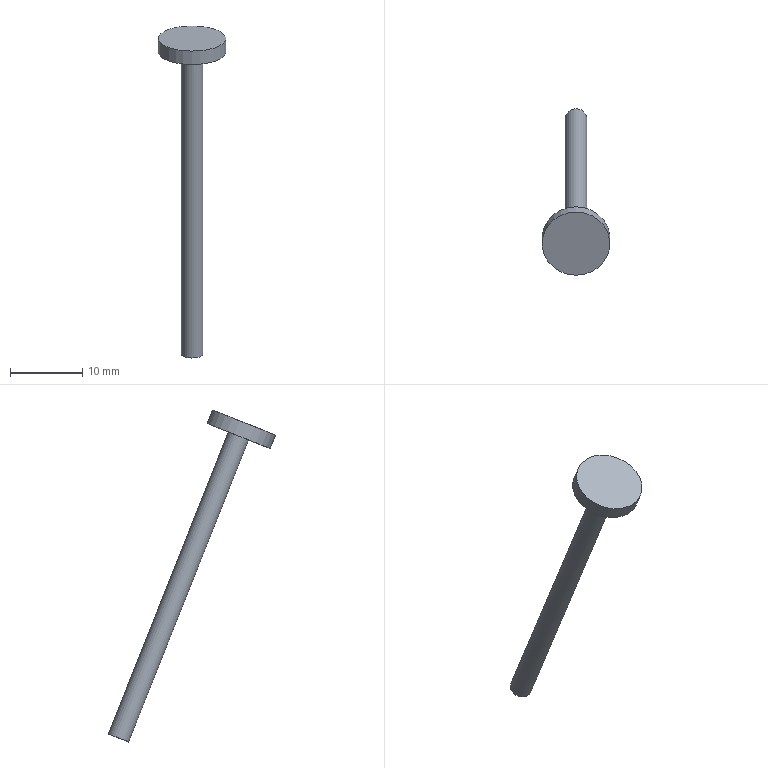Part | STEP file | Revolve1 | 1 solid | 5 faces | box 9.4 x 23.118 x 45.968 mm | volume 456.882 mm3 | plane 3 | cylinder 2 | commonest cylinder face diameters 3 x1 9.4 x1
STEP:
#1=CARTESIAN_POINT('',(0.,0.,0.));
#2=DIRECTION('',(0.,0.,1.));
#3=DIRECTION('',(1.,0.,0.));
#4=AXIS2_PLACEMENT_3D('',#1,#2,#3);
#5=CARTESIAN_POINT('',(140.817,148.133,-138.172));
#6=VERTEX_POINT('',#5);
#7=CARTESIAN_POINT('',(140.817,131.516,-96.352));
#8=VERTEX_POINT('',#7);
#9=CARTESIAN_POINT('',(140.817,148.133,-138.172));
#10=DIRECTION('',(0.,-0.3693,0.9293));
#11=VECTOR('',#10,1.);
#12=LINE('',#9,#11);
#13=CARTESIAN_POINT('',(140.797,130.122,-96.906));
#14=DIRECTION('',(0.,0.3693,-0.9293));
#15=DIRECTION('',(0.01361,0.9292,0.3692));
#16=AXIS2_PLACEMENT_3D('',#13,#14,#15);
#17=CYLINDRICAL_SURFACE('',#16,1.5);
#18=CARTESIAN_POINT('',(0.000000001,45.));
#19=DIRECTION('',(0.,-1.));
#20=VECTOR('',#19,1.);
#21=LINE('',#18,#20);
#22=(GEOMETRIC_REPRESENTATION_CONTEXT(2)PARAMETRIC_REPRESENTATION_CONTEXT()REPRESENTATION_CONTEXT('',''));
#23=DEFINITIONAL_REPRESENTATION('',(#21),#22);
#24=PCURVE('',#17,#23);
#25=CARTESIAN_POINT('',(6.283,45.));
#26=DIRECTION('',(0.,-1.));
#27=VECTOR('',#26,1.);
#28=LINE('',#25,#27);
#29=(GEOMETRIC_REPRESENTATION_CONTEXT(2)PARAMETRIC_REPRESENTATION_CONTEXT()REPRESENTATION_CONTEXT('',''));
#30=DEFINITIONAL_REPRESENTATION('',(#28),#29);
#31=PCURVE('',#17,#30);
#32=SEAM_CURVE('',#12,(#24,#31),.PCURVE_S1.);
#33=EDGE_CURVE('',#6,#8,#32,.T.);
#34=ORIENTED_EDGE('',*,*,#33,.T.);
#35=CARTESIAN_POINT('',(140.797,130.122,-96.906));
#36=DIRECTION('',(0.,0.3693,-0.9293));
#37=DIRECTION('',(0.01361,0.9292,0.3692));
#38=AXIS2_PLACEMENT_3D('',#35,#36,#37);
#39=CIRCLE('',#38,1.5);
#40=CARTESIAN_POINT('',(0.,0.));
#41=DIRECTION('',(1.,0.));
#42=VECTOR('',#41,1.);
#43=LINE('',#40,#42);
#44=(GEOMETRIC_REPRESENTATION_CONTEXT(2)PARAMETRIC_REPRESENTATION_CONTEXT()REPRESENTATION_CONTEXT('',''));
#45=DEFINITIONAL_REPRESENTATION('',(#43),#44);
#46=PCURVE('',#17,#45);
#47=CARTESIAN_POINT('',(140.797,130.122,-96.906));
#48=DIRECTION('',(0.,-0.3693,0.9293));
#49=DIRECTION('',(-0.01361,-0.9292,-0.3692));
#50=AXIS2_PLACEMENT_3D('',#47,#48,#49);
#51=PLANE('',#50);
#52=CARTESIAN_POINT('',(-1.5,0.));
#53=CARTESIAN_POINT('',(-1.5,2.598));
#54=CARTESIAN_POINT('',(0.75,1.299));
#55=CARTESIAN_POINT('',(3.,0.));
#56=CARTESIAN_POINT('',(0.75,-1.299));
#57=CARTESIAN_POINT('',(-1.5,-2.598));
#58=CARTESIAN_POINT('',(-1.5,0.));
#59=(BOUNDED_CURVE()B_SPLINE_CURVE(2,(#52,#53,#54,#55,#56,#57,#58),.UNSPECIFIED.,.T.,.F.)B_SPLINE_CURVE_WITH_KNOTS((1,2,2,2,2,1),(-2.094,0.,2.094,4.189,6.283,8.378),.UNSPECIFIED.)CURVE()GEOMETRIC_REPRESENTATION_ITEM()RATIONAL_B_SPLINE_CURVE((1.,0.5,1.,0.5,1.,0.5,1.))REPRESENTATION_ITEM(''));
#60=(GEOMETRIC_REPRESENTATION_CONTEXT(2)PARAMETRIC_REPRESENTATION_CONTEXT()REPRESENTATION_CONTEXT('',''));
#61=DEFINITIONAL_REPRESENTATION('',(#59),#60);
#62=PCURVE('',#51,#61);
#63=SURFACE_CURVE('',#39,(#46,#62),.PCURVE_S1.);
#64=EDGE_CURVE('',#8,#8,#63,.T.);
#65=ORIENTED_EDGE('',*,*,#64,.T.);
#66=ORIENTED_EDGE('',*,*,#33,.F.);
#67=CARTESIAN_POINT('',(140.797,146.739,-138.726));
#68=DIRECTION('',(0.,-0.3693,0.9293));
#69=DIRECTION('',(0.01361,0.9292,0.3692));
#70=AXIS2_PLACEMENT_3D('',#67,#68,#69);
#71=CIRCLE('',#70,1.5);
#72=CARTESIAN_POINT('',(6.283,45.));
#73=DIRECTION('',(-1.,0.));
#74=VECTOR('',#73,1.);
#75=LINE('',#72,#74);
#76=(GEOMETRIC_REPRESENTATION_CONTEXT(2)PARAMETRIC_REPRESENTATION_CONTEXT()REPRESENTATION_CONTEXT('',''));
#77=DEFINITIONAL_REPRESENTATION('',(#75),#76);
#78=PCURVE('',#17,#77);
#79=CARTESIAN_POINT('',(140.797,146.739,-138.726));
#80=DIRECTION('',(0.,-0.3693,0.9293));
#81=DIRECTION('',(-0.01361,-0.9292,-0.3692));
#82=AXIS2_PLACEMENT_3D('',#79,#80,#81);
#83=PLANE('',#82);
#84=CARTESIAN_POINT('',(0.,0.));
#85=DIRECTION('',(-1.,0.));
#86=AXIS2_PLACEMENT_2D('',#84,#85);
#87=CIRCLE('',#86,1.5);
#88=(GEOMETRIC_REPRESENTATION_CONTEXT(2)PARAMETRIC_REPRESENTATION_CONTEXT()REPRESENTATION_CONTEXT('',''));
#89=DEFINITIONAL_REPRESENTATION('',(#87),#88);
#90=PCURVE('',#83,#89);
#91=SURFACE_CURVE('',#71,(#78,#90),.PCURVE_S1.);
#92=EDGE_CURVE('',#6,#6,#91,.T.);
#93=ORIENTED_EDGE('',*,*,#92,.T.);
#94=EDGE_LOOP('',(#34,#65,#66,#93));
#95=FACE_BOUND('',#94,.T.);
#96=ADVANCED_FACE('',(#95),#17,.T.);
#97=CARTESIAN_POINT('',(140.861,134.489,-95.171));
#98=VERTEX_POINT('',#97);
#99=CARTESIAN_POINT('',(140.861,133.751,-93.312));
#100=VERTEX_POINT('',#99);
#101=CARTESIAN_POINT('',(140.861,134.489,-95.171));
#102=DIRECTION('',(0.,-0.3693,0.9293));
#103=VECTOR('',#102,1.);
#104=LINE('',#101,#103);
#105=CARTESIAN_POINT('',(140.797,129.383,-95.048));
#106=DIRECTION('',(0.,0.3693,-0.9293));
#107=DIRECTION('',(0.01361,0.9292,0.3692));
#108=AXIS2_PLACEMENT_3D('',#105,#106,#107);
#109=CYLINDRICAL_SURFACE('',#108,4.7);
#110=CARTESIAN_POINT('',(0.,2.));
#111=DIRECTION('',(0.,-1.));
#112=VECTOR('',#111,1.);
#113=LINE('',#110,#112);
#114=(GEOMETRIC_REPRESENTATION_CONTEXT(2)PARAMETRIC_REPRESENTATION_CONTEXT()REPRESENTATION_CONTEXT('',''));
#115=DEFINITIONAL_REPRESENTATION('',(#113),#114);
#116=PCURVE('',#109,#115);
#117=CARTESIAN_POINT('',(6.283,2.));
#118=DIRECTION('',(0.,-1.));
#119=VECTOR('',#118,1.);
#120=LINE('',#117,#119);
#121=(GEOMETRIC_REPRESENTATION_CONTEXT(2)PARAMETRIC_REPRESENTATION_CONTEXT()REPRESENTATION_CONTEXT('',''));
#122=DEFINITIONAL_REPRESENTATION('',(#120),#121);
#123=PCURVE('',#109,#122);
#124=SEAM_CURVE('',#104,(#116,#123),.PCURVE_S1.);
#125=EDGE_CURVE('',#98,#100,#124,.T.);
#126=ORIENTED_EDGE('',*,*,#125,.T.);
#127=CARTESIAN_POINT('',(140.797,129.383,-95.048));
#128=DIRECTION('',(0.,0.3693,-0.9293));
#129=DIRECTION('',(0.01361,0.9292,0.3692));
#130=AXIS2_PLACEMENT_3D('',#127,#128,#129);
#131=CIRCLE('',#130,4.7);
#132=CARTESIAN_POINT('',(0.,0.));
#133=DIRECTION('',(1.,0.));
#134=VECTOR('',#133,1.);
#135=LINE('',#132,#134);
#136=(GEOMETRIC_REPRESENTATION_CONTEXT(2)PARAMETRIC_REPRESENTATION_CONTEXT()REPRESENTATION_CONTEXT('',''));
#137=DEFINITIONAL_REPRESENTATION('',(#135),#136);
#138=PCURVE('',#109,#137);
#139=CARTESIAN_POINT('',(140.797,129.383,-95.048));
#140=DIRECTION('',(0.,0.3693,-0.9293));
#141=DIRECTION('',(0.01361,0.9292,0.3692));
#142=AXIS2_PLACEMENT_3D('',#139,#140,#141);
#143=PLANE('',#142);
#144=CARTESIAN_POINT('',(0.,0.));
#145=DIRECTION('',(1.,0.));
#146=AXIS2_PLACEMENT_2D('',#144,#145);
#147=CIRCLE('',#146,4.7);
#148=(GEOMETRIC_REPRESENTATION_CONTEXT(2)PARAMETRIC_REPRESENTATION_CONTEXT()REPRESENTATION_CONTEXT('',''));
#149=DEFINITIONAL_REPRESENTATION('',(#147),#148);
#150=PCURVE('',#143,#149);
#151=SURFACE_CURVE('',#131,(#138,#150),.PCURVE_S1.);
#152=EDGE_CURVE('',#100,#100,#151,.T.);
#153=ORIENTED_EDGE('',*,*,#152,.T.);
#154=ORIENTED_EDGE('',*,*,#125,.F.);
#155=CARTESIAN_POINT('',(140.797,130.122,-96.906));
#156=DIRECTION('',(0.,-0.3693,0.9293));
#157=DIRECTION('',(0.01361,0.9292,0.3692));
#158=AXIS2_PLACEMENT_3D('',#155,#156,#157);
#159=CIRCLE('',#158,4.7);
#160=CARTESIAN_POINT('',(6.283,2.));
#161=DIRECTION('',(-1.,0.));
#162=VECTOR('',#161,1.);
#163=LINE('',#160,#162);
#164=(GEOMETRIC_REPRESENTATION_CONTEXT(2)PARAMETRIC_REPRESENTATION_CONTEXT()REPRESENTATION_CONTEXT('',''));
#165=DEFINITIONAL_REPRESENTATION('',(#163),#164);
#166=PCURVE('',#109,#165);
#167=CARTESIAN_POINT('',(0.,0.));
#168=DIRECTION('',(-1.,0.));
#169=AXIS2_PLACEMENT_2D('',#167,#168);
#170=CIRCLE('',#169,4.7);
#171=(GEOMETRIC_REPRESENTATION_CONTEXT(2)PARAMETRIC_REPRESENTATION_CONTEXT()REPRESENTATION_CONTEXT('',''));
#172=DEFINITIONAL_REPRESENTATION('',(#170),#171);
#173=PCURVE('',#51,#172);
#174=SURFACE_CURVE('',#159,(#166,#173),.PCURVE_S1.);
#175=EDGE_CURVE('',#98,#98,#174,.T.);
#176=ORIENTED_EDGE('',*,*,#175,.T.);
#177=EDGE_LOOP('',(#126,#153,#154,#176));
#178=FACE_BOUND('',#177,.T.);
#179=ADVANCED_FACE('',(#178),#109,.T.);
#180=ORIENTED_EDGE('',*,*,#64,.F.);
#181=EDGE_LOOP('',(#180));
#182=FACE_BOUND('',#181,.T.);
#183=ORIENTED_EDGE('',*,*,#175,.F.);
#184=EDGE_LOOP('',(#183));
#185=FACE_BOUND('',#184,.T.);
#186=ADVANCED_FACE('',(#182,#185),#51,.F.);
#187=ORIENTED_EDGE('',*,*,#92,.F.);
#188=EDGE_LOOP('',(#187));
#189=FACE_BOUND('',#188,.T.);
#190=ADVANCED_FACE('',(#189),#83,.F.);
#191=ORIENTED_EDGE('',*,*,#152,.F.);
#192=EDGE_LOOP('',(#191));
#193=FACE_BOUND('',#192,.T.);
#194=ADVANCED_FACE('',(#193),#143,.F.);
#195=CLOSED_SHELL('',(#96,#179,#186,#190,#194));
#196=MANIFOLD_SOLID_BREP('',#195);
#197=(LENGTH_UNIT()NAMED_UNIT(*)SI_UNIT(.MILLI.,.METRE.));
#198=UNCERTAINTY_MEASURE_WITH_UNIT(LENGTH_MEASURE(0.0000001),#197,'','');
#199=(NAMED_UNIT(*)PLANE_ANGLE_UNIT()SI_UNIT($,.RADIAN.));
#200=(NAMED_UNIT(*)SI_UNIT($,.STERADIAN.)SOLID_ANGLE_UNIT());
#201=(GEOMETRIC_REPRESENTATION_CONTEXT(3)GLOBAL_UNCERTAINTY_ASSIGNED_CONTEXT((#198))GLOBAL_UNIT_ASSIGNED_CONTEXT((#197,#199,#200))REPRESENTATION_CONTEXT('',''));
#202=ADVANCED_BREP_SHAPE_REPRESENTATION('',(#4,#196),#201);